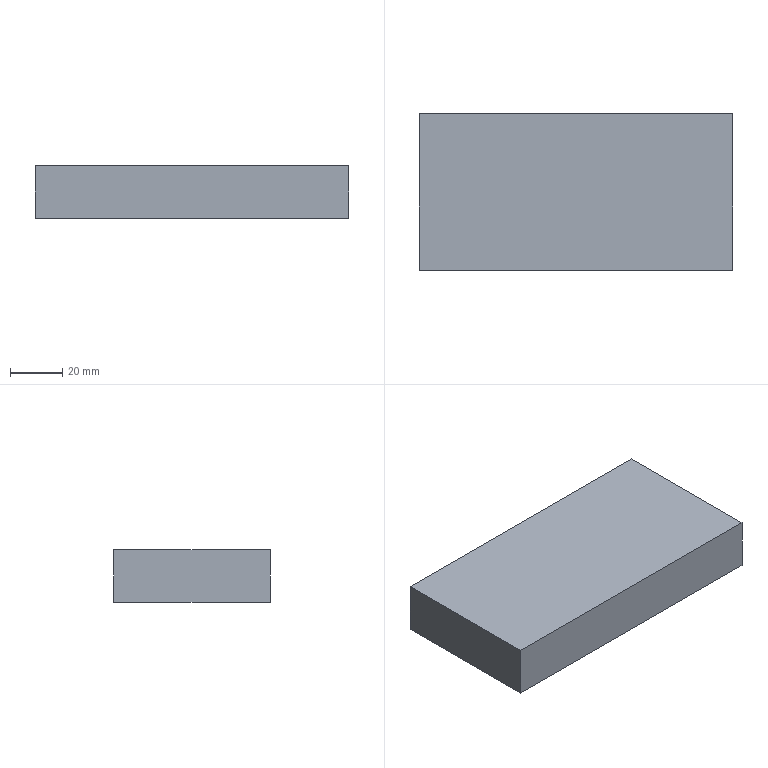Part | SolidWorks | features Extrusion 1 | 1 solid | 6 faces | box 120 x 60 x 20 mm | volume 144000 mm3 | plane 6
STEP:
#1=CARTESIAN_POINT('',(0.,60.,0.));
#2=VERTEX_POINT('',#1);
#3=CARTESIAN_POINT('',(0.,0.,0.));
#4=VERTEX_POINT('',#3);
#5=CARTESIAN_POINT('',(0.,0.,0.));
#6=DIRECTION('',(0.,-1.,0.));
#7=VECTOR('',#6,1000.);
#8=LINE('',#5,#7);
#9=EDGE_CURVE('',#2,#4,#8,.T.);
#10=ORIENTED_EDGE('',*,*,#9,.T.);
#11=CARTESIAN_POINT('',(0.,0.,20.));
#12=VERTEX_POINT('',#11);
#13=CARTESIAN_POINT('',(0.,0.,20.));
#14=DIRECTION('',(0.,0.,-1.));
#15=VECTOR('',#14,1000.);
#16=LINE('',#13,#15);
#17=EDGE_CURVE('',#12,#4,#16,.T.);
#18=ORIENTED_EDGE('',*,*,#17,.F.);
#19=CARTESIAN_POINT('',(0.,60.,20.));
#20=VERTEX_POINT('',#19);
#21=CARTESIAN_POINT('',(0.,0.,20.));
#22=DIRECTION('',(0.,-1.,0.));
#23=VECTOR('',#22,1000.);
#24=LINE('',#21,#23);
#25=EDGE_CURVE('',#20,#12,#24,.T.);
#26=ORIENTED_EDGE('',*,*,#25,.F.);
#27=CARTESIAN_POINT('',(0.,60.,20.));
#28=DIRECTION('',(0.,0.,-1.));
#29=VECTOR('',#28,1000.);
#30=LINE('',#27,#29);
#31=EDGE_CURVE('',#20,#2,#30,.T.);
#32=ORIENTED_EDGE('',*,*,#31,.T.);
#33=EDGE_LOOP('',(#10,#18,#26,#32));
#34=FACE_OUTER_BOUND('',#33,.T.);
#35=CARTESIAN_POINT('',(0.,0.,20.));
#36=DIRECTION('',(1.,0.,0.));
#37=DIRECTION('',(0.,0.,-1.));
#38=AXIS2_PLACEMENT_3D('',#35,#36,#37);
#39=PLANE('',#38);
#40=ADVANCED_FACE('',(#34),#39,.F.);
#41=CARTESIAN_POINT('',(120.,0.,0.));
#42=VERTEX_POINT('',#41);
#43=CARTESIAN_POINT('',(0.,0.,0.));
#44=DIRECTION('',(1.,0.,0.));
#45=VECTOR('',#44,1000.);
#46=LINE('',#43,#45);
#47=EDGE_CURVE('',#4,#42,#46,.T.);
#48=ORIENTED_EDGE('',*,*,#47,.T.);
#49=CARTESIAN_POINT('',(120.,0.,20.));
#50=VERTEX_POINT('',#49);
#51=CARTESIAN_POINT('',(120.,0.,20.));
#52=DIRECTION('',(0.,0.,-1.));
#53=VECTOR('',#52,1000.);
#54=LINE('',#51,#53);
#55=EDGE_CURVE('',#50,#42,#54,.T.);
#56=ORIENTED_EDGE('',*,*,#55,.F.);
#57=CARTESIAN_POINT('',(0.,0.,20.));
#58=DIRECTION('',(1.,0.,0.));
#59=VECTOR('',#58,1000.);
#60=LINE('',#57,#59);
#61=EDGE_CURVE('',#12,#50,#60,.T.);
#62=ORIENTED_EDGE('',*,*,#61,.F.);
#63=ORIENTED_EDGE('',*,*,#17,.T.);
#64=EDGE_LOOP('',(#48,#56,#62,#63));
#65=FACE_OUTER_BOUND('',#64,.T.);
#66=CARTESIAN_POINT('',(0.,0.,20.));
#67=DIRECTION('',(0.,1.,0.));
#68=DIRECTION('',(0.,0.,1.));
#69=AXIS2_PLACEMENT_3D('',#66,#67,#68);
#70=PLANE('',#69);
#71=ADVANCED_FACE('',(#65),#70,.F.);
#72=CARTESIAN_POINT('',(120.,60.,0.));
#73=VERTEX_POINT('',#72);
#74=CARTESIAN_POINT('',(120.,0.,0.));
#75=DIRECTION('',(0.,1.,0.));
#76=VECTOR('',#75,1000.);
#77=LINE('',#74,#76);
#78=EDGE_CURVE('',#42,#73,#77,.T.);
#79=ORIENTED_EDGE('',*,*,#78,.T.);
#80=CARTESIAN_POINT('',(120.,60.,20.));
#81=VERTEX_POINT('',#80);
#82=CARTESIAN_POINT('',(120.,60.,20.));
#83=DIRECTION('',(0.,0.,-1.));
#84=VECTOR('',#83,1000.);
#85=LINE('',#82,#84);
#86=EDGE_CURVE('',#81,#73,#85,.T.);
#87=ORIENTED_EDGE('',*,*,#86,.F.);
#88=CARTESIAN_POINT('',(120.,0.,20.));
#89=DIRECTION('',(0.,1.,0.));
#90=VECTOR('',#89,1000.);
#91=LINE('',#88,#90);
#92=EDGE_CURVE('',#50,#81,#91,.T.);
#93=ORIENTED_EDGE('',*,*,#92,.F.);
#94=ORIENTED_EDGE('',*,*,#55,.T.);
#95=EDGE_LOOP('',(#79,#87,#93,#94));
#96=FACE_OUTER_BOUND('',#95,.T.);
#97=CARTESIAN_POINT('',(120.,0.,20.));
#98=DIRECTION('',(-1.,0.,0.));
#99=DIRECTION('',(0.,0.,1.));
#100=AXIS2_PLACEMENT_3D('',#97,#98,#99);
#101=PLANE('',#100);
#102=ADVANCED_FACE('',(#96),#101,.F.);
#103=CARTESIAN_POINT('',(0.,60.,0.));
#104=DIRECTION('',(-1.,0.,0.));
#105=VECTOR('',#104,1000.);
#106=LINE('',#103,#105);
#107=EDGE_CURVE('',#73,#2,#106,.T.);
#108=ORIENTED_EDGE('',*,*,#107,.T.);
#109=ORIENTED_EDGE('',*,*,#31,.F.);
#110=CARTESIAN_POINT('',(0.,60.,20.));
#111=DIRECTION('',(-1.,0.,0.));
#112=VECTOR('',#111,1000.);
#113=LINE('',#110,#112);
#114=EDGE_CURVE('',#81,#20,#113,.T.);
#115=ORIENTED_EDGE('',*,*,#114,.F.);
#116=ORIENTED_EDGE('',*,*,#86,.T.);
#117=EDGE_LOOP('',(#108,#109,#115,#116));
#118=FACE_OUTER_BOUND('',#117,.T.);
#119=CARTESIAN_POINT('',(0.,60.,20.));
#120=DIRECTION('',(0.,-1.,0.));
#121=DIRECTION('',(0.,0.,-1.));
#122=AXIS2_PLACEMENT_3D('',#119,#120,#121);
#123=PLANE('',#122);
#124=ADVANCED_FACE('',(#118),#123,.F.);
#125=ORIENTED_EDGE('',*,*,#25,.T.);
#126=ORIENTED_EDGE('',*,*,#61,.T.);
#127=ORIENTED_EDGE('',*,*,#92,.T.);
#128=ORIENTED_EDGE('',*,*,#114,.T.);
#129=EDGE_LOOP('',(#125,#126,#127,#128));
#130=FACE_OUTER_BOUND('',#129,.T.);
#131=CARTESIAN_POINT('',(0.,0.,20.));
#132=DIRECTION('',(0.,0.,-1.));
#133=DIRECTION('',(-1.,0.,0.));
#134=AXIS2_PLACEMENT_3D('',#131,#132,#133);
#135=PLANE('',#134);
#136=ADVANCED_FACE('',(#130),#135,.F.);
#137=ORIENTED_EDGE('',*,*,#9,.F.);
#138=ORIENTED_EDGE('',*,*,#107,.F.);
#139=ORIENTED_EDGE('',*,*,#78,.F.);
#140=ORIENTED_EDGE('',*,*,#47,.F.);
#141=EDGE_LOOP('',(#137,#138,#139,#140));
#142=FACE_OUTER_BOUND('',#141,.T.);
#143=CARTESIAN_POINT('',(0.,0.,0.));
#144=DIRECTION('',(0.,0.,-1.));
#145=DIRECTION('',(-1.,0.,0.));
#146=AXIS2_PLACEMENT_3D('',#143,#144,#145);
#147=PLANE('',#146);
#148=ADVANCED_FACE('',(#142),#147,.T.);
#149=CLOSED_SHELL('',(#40,#71,#102,#124,#136,#148));
#150=MANIFOLD_SOLID_BREP('',#149);
#151=CARTESIAN_POINT('',(0.,0.,0.));
#152=DIRECTION('',(0.,0.,1.));
#153=DIRECTION('',(1.,0.,0.));
#154=AXIS2_PLACEMENT_3D('',#151,#152,#153);
#155=(LENGTH_UNIT()NAMED_UNIT(*)SI_UNIT(.MILLI.,.METRE.));
#156=UNCERTAINTY_MEASURE_WITH_UNIT(LENGTH_MEASURE(0.00001),#155,'','');
#157=(NAMED_UNIT(*)PLANE_ANGLE_UNIT()SI_UNIT($,.RADIAN.));
#158=(NAMED_UNIT(*)SI_UNIT($,.STERADIAN.)SOLID_ANGLE_UNIT());
#159=(GEOMETRIC_REPRESENTATION_CONTEXT(3)GLOBAL_UNCERTAINTY_ASSIGNED_CONTEXT((#156))GLOBAL_UNIT_ASSIGNED_CONTEXT((#155,#157,#158))REPRESENTATION_CONTEXT('',''));
#160=ADVANCED_BREP_SHAPE_REPRESENTATION('',(#150,#154),#159);